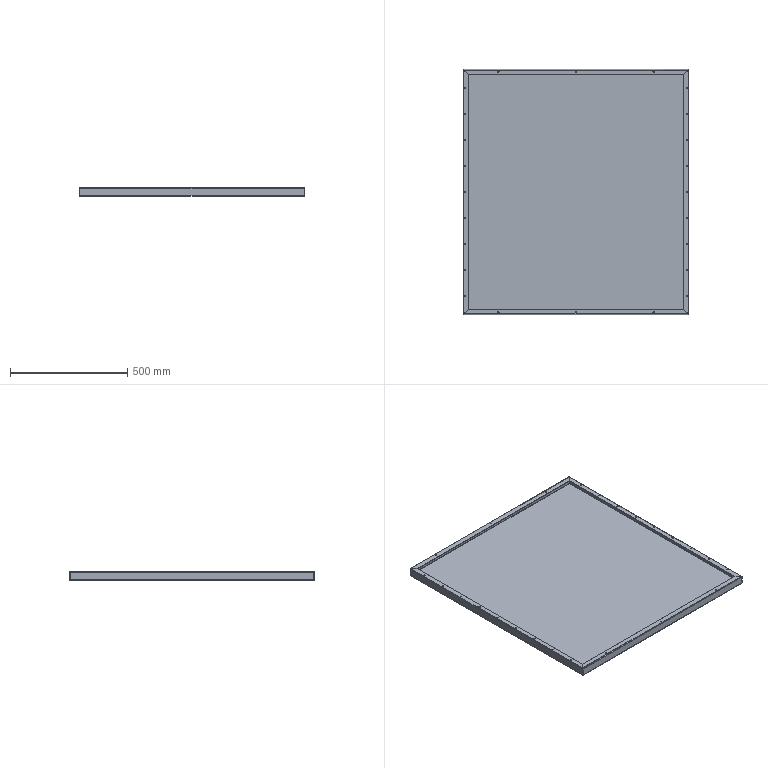Part | SolidWorks | 1 solid | 118 faces | box 962 x 1043 x 37 mm | volume 3028996 mm3 | cylinder 64 | plane 38 | spline 16 | commonest cylinder face diameters 5 x48 1.473 x8 6.473 x8